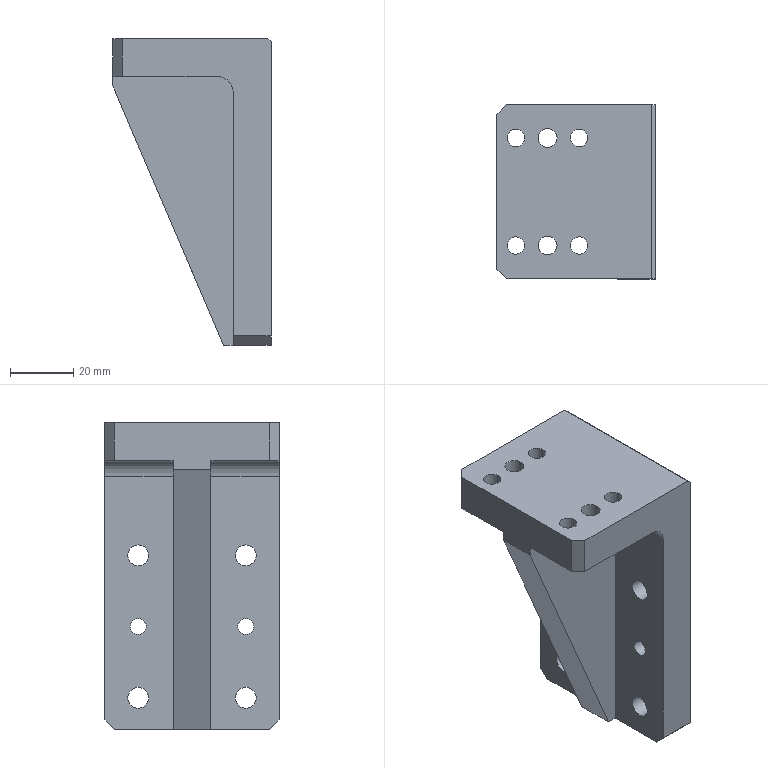CAM job | NX | 3+2 milling, drilling | part box 50 x 55 x 97 mm | stock box 55 x 60 x 102 mm
Tools:
number,name,description,diameter,corner_radius,flute_length,length,flutes
9,D10,平底铣刀-粗,10.0,0.0,35.0,75.0,2
7,D6-J,平底铣刀-精,6.0,0.0,25.0,75.0,2
10,D10-J,平底铣刀-精,10.0,0.0,35.0,75.0,2
17,D6R0.5,圆鼻刀-粗,6.0,0.5,50.0,75.0,2
1,D80R0.8飞刀,圆鼻刀-粗,80.0,0.8,50.0,75.0,2
1,D80R0.8飞刀-J,圆鼻刀-精,80.0,0.8,50.0,75.0,2
2,D6倒角刀,倒角刀,6.0,0.0,3.0,25.0,2
19,D5铰刀,Drilling Tool,5.0,0.0,75.0,100.0,6
18,钻头6.6,Drilling Tool,6.6,0.0,35.0,50.0,2
17,ZT4.9,Drilling Tool,4.9,0.0,35.0,50.0,2
Operations:
program,operation,operation_type,tool,method,geometry_group,spindle_rpm,surface_speed,feed_per_tooth,feed_cut,feed_plunge,cut_length_mm,path_length_mm,cut_time_min,machine_time_min
B,FLOORWALLFLYFACEONEPASSROUGH_COPY,VolumeBased25DMillingOperation,D80R0.8飞刀,分层开粗-切深K-步距G,W-B,2800.0,703.696,0.5357,3000.0,100.0,1846.746,4014.966,0.6156,0.8324
B,FLOORWALLFLYFACEONEPASSFINISH_COPY,VolumeBased25DMillingOperation,D80R0.8飞刀-J,侧刃精光-切深K-步距G,W-B,4000.0,1005.28,0.125,1000.0,100.0,204.998,300.998,0.205,0.2146
B,CAVITYROUGH-MID_COPY,CavityMilling,D10,分层开粗-切深K-步距G,W-B,8000.0,251.32,0.25,4000.0,100.0,60906.674,64093.265,15.227,15.693
B,ZLEVELFINISHSTEEPZIGZAG_COPY,ZLevelMilling,D6R0.5,等高爬面-切深K-步距G,W-B,8000.0,150.796,0.2188,3500.0,100.0,1236.984,1357.86,0.3534,0.3655
B,ZLEVELFINISHSTEEPZIGZAG_COPY_COPY,ZLevelMilling,D6R0.5,等高爬面-切深K-步距G,W-B,8000.0,150.796,0.2188,3500.0,100.0,12912.489,12976.477,3.689,3.696
B,PLANARDEBURR6X45L_COPY,SurfaceContour,D6倒角刀,STEEPCHAMFER-DEPTH0-STEPG,W-B,6500.0,122.519,0.1154,1500.0,100.0,411.175,1564.396,0.2741,0.3894
B,FLOORWALLFINISHFLOOR-MID_COPY,VolumeBased25DMillingOperation,D6-J,精光步距切深关,W-B,7000.0,175.0,0.0536,1500.0,100.0,1268.407,1524.561,0.8456,0.8712
B,ZLEVELFINISH-MID_COPY,ZLevelMilling,D6-J,侧刃精光-切深K-步距G,W-B,8000.0,150.792,0.0625,1000.0,100.0,1017.801,1845.588,1.018,1.101
B,ZLEVELFINISHSTEEPZIGZAG_COPY_COPY_COPY,ZLevelMilling,D6-J,等高爬面-切深K-步距G,W-B,8000.0,150.796,0.2188,3500.0,100.0,19076.372,19321.511,5.45,5.475
A,TOPFACE,FaceMilling,D80R0.8飞刀,侧刃精光-切深K-步距G,W-A,4500.0,1385.0,0.1667,1500.0,100.0,191.0,287.0,0.1273,0.1369
A,PROFILE-ROUGH_2,VolumeBased25DMillingOperation,D10,METHOD,W-A,8000.0,251.327,0.375,6000.0,80.0,21615.979,21764.479,3.603,3.618
A,SPOTDRILL-DEPTH0.8,Operation,D6倒角刀,NONE,W-A,8000.0,150.796,0.0312,500.0,90.0,10.8,250.703,0.0216,0.0456
A,THRUHOLE-FINISH6.0-PREDRILL,Operation,ZT4.9,NONE,W-A,2500.0,38.484,0.05,250.0,90.0,34.829,204.673,0.1393,0.1563
A,THRUHOLE-6-8,Operation,钻头6.6,NONE,W-A,2500.0,51.836,0.03,150.0,90.0,67.621,351.283,0.4508,0.4792
A,SELECTBODYONLY,SurfaceContour,D6倒角刀,METHOD,W-A,8000.0,150.796,0.1875,3000.0,100.0,257.378,351.509,0.0858,0.0952
A,MILLCHAMFER_1,PlanarMilling,D6倒角刀,METHOD,W-A,8000.0,150.796,0.0312,500.0,100.0,36.963,274.532,0.0739,0.0977
A,MILLCHAMFER_2,PlanarMilling,D6倒角刀,METHOD,W-A,8000.0,150.796,0.05,800.0,100.0,92.54,609.64,0.1157,0.1674
A,FLOORWALLCHAMFER_COPY,VolumeBased25DMillingOperation,D6倒角刀,STEEPCHAMFER-DEPTH0-STEPG,W-A,6500.0,122.519,0.1154,1500.0,100.0,63.801,164.201,0.0425,0.0526
A,REAMING,Operation,D5铰刀,METHOD,W-A,500.0,7.854,0.0167,50.0,0.0,28.0,191.015,0.56,0.5763
A,PROFILE-SEMIFINISH_2,VolumeBased25DMillingOperation,D10-J,METHOD,W-A,9000.0,169.646,0.0667,1200.0,100.0,1684.297,2489.355,1.404,1.484